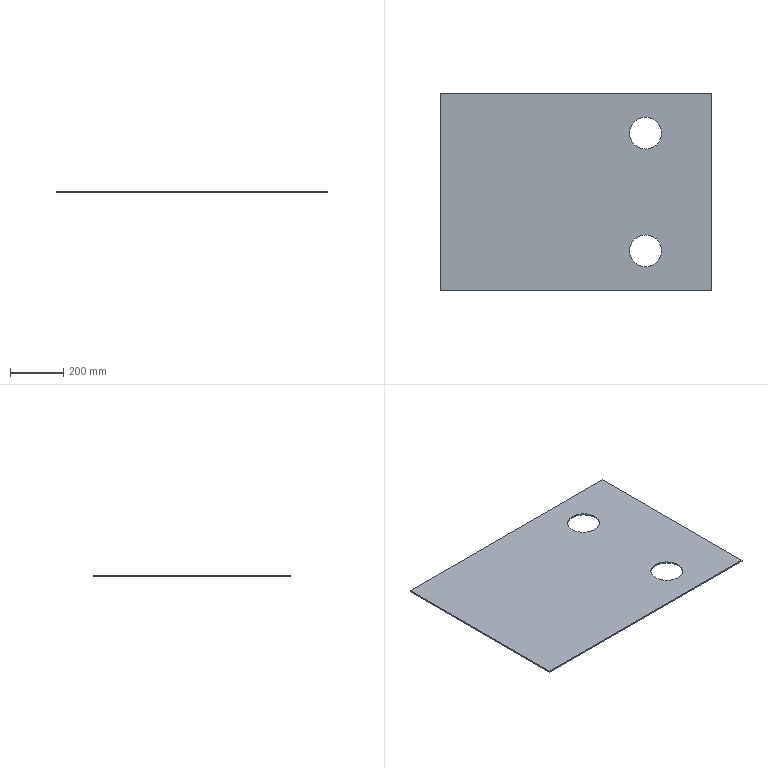Part | SolidWorks | features BaseBody 1 | 1 solid | 10 faces | box 1023 x 743 x 5 mm | volume 3687348 mm3 | plane 6 | cylinder 4 | commonest cylinder face diameters 120 x4
STEP:
#1=CARTESIAN_POINT('',(-250.,653.,5.));
#2=VERTEX_POINT('',#1);
#3=CARTESIAN_POINT('',(-250.,533.,5.));
#4=VERTEX_POINT('',#3);
#5=CARTESIAN_POINT('',(-250.,593.,5.));
#6=DIRECTION('',(0.,0.,1.));
#7=DIRECTION('',(0.,1.,0.));
#8=AXIS2_PLACEMENT_3D('',#5,#6,#7);
#9=CIRCLE('',#8,60.);
#10=EDGE_CURVE('',#2,#4,#9,.T.);
#11=ORIENTED_EDGE('',*,*,#10,.T.);
#12=CARTESIAN_POINT('',(-250.,533.,0.));
#13=VERTEX_POINT('',#12);
#14=CARTESIAN_POINT('',(-250.,533.,5.));
#15=DIRECTION('',(0.,0.,-1.));
#16=VECTOR('',#15,1000.);
#17=LINE('',#14,#16);
#18=EDGE_CURVE('',#4,#13,#17,.T.);
#19=ORIENTED_EDGE('',*,*,#18,.T.);
#20=CARTESIAN_POINT('',(-250.,653.,0.));
#21=VERTEX_POINT('',#20);
#22=CARTESIAN_POINT('',(-250.,593.,0.));
#23=DIRECTION('',(0.,0.,-1.));
#24=DIRECTION('',(0.,1.,0.));
#25=AXIS2_PLACEMENT_3D('',#22,#23,#24);
#26=CIRCLE('',#25,60.);
#27=EDGE_CURVE('',#13,#21,#26,.T.);
#28=ORIENTED_EDGE('',*,*,#27,.T.);
#29=CARTESIAN_POINT('',(-250.,653.,5.));
#30=DIRECTION('',(0.,0.,-1.));
#31=VECTOR('',#30,1000.);
#32=LINE('',#29,#31);
#33=EDGE_CURVE('',#2,#21,#32,.T.);
#34=ORIENTED_EDGE('',*,*,#33,.F.);
#35=EDGE_LOOP('',(#11,#19,#28,#34));
#36=FACE_OUTER_BOUND('',#35,.T.);
#37=CARTESIAN_POINT('',(-250.,593.,5.));
#38=DIRECTION('',(0.,0.,-1.));
#39=DIRECTION('',(0.,1.,0.));
#40=AXIS2_PLACEMENT_3D('',#37,#38,#39);
#41=CYLINDRICAL_SURFACE('',#40,60.);
#42=ADVANCED_FACE('',(#36),#41,.F.);
#43=CARTESIAN_POINT('',(-250.,90.,5.));
#44=VERTEX_POINT('',#43);
#45=CARTESIAN_POINT('',(-250.,210.,5.));
#46=VERTEX_POINT('',#45);
#47=CARTESIAN_POINT('',(-250.,150.,5.));
#48=DIRECTION('',(0.,0.,-1.));
#49=DIRECTION('',(0.,1.,0.));
#50=AXIS2_PLACEMENT_3D('',#47,#48,#49);
#51=CIRCLE('',#50,60.);
#52=EDGE_CURVE('',#44,#46,#51,.T.);
#53=ORIENTED_EDGE('',*,*,#52,.F.);
#54=CARTESIAN_POINT('',(-250.,90.,0.));
#55=VERTEX_POINT('',#54);
#56=CARTESIAN_POINT('',(-250.,90.,5.));
#57=DIRECTION('',(0.,0.,-1.));
#58=VECTOR('',#57,1000.);
#59=LINE('',#56,#58);
#60=EDGE_CURVE('',#44,#55,#59,.T.);
#61=ORIENTED_EDGE('',*,*,#60,.T.);
#62=CARTESIAN_POINT('',(-250.,210.,0.));
#63=VERTEX_POINT('',#62);
#64=CARTESIAN_POINT('',(-250.,150.,0.));
#65=DIRECTION('',(0.,0.,-1.));
#66=DIRECTION('',(0.,1.,0.));
#67=AXIS2_PLACEMENT_3D('',#64,#65,#66);
#68=CIRCLE('',#67,60.);
#69=EDGE_CURVE('',#55,#63,#68,.T.);
#70=ORIENTED_EDGE('',*,*,#69,.T.);
#71=CARTESIAN_POINT('',(-250.,210.,5.));
#72=DIRECTION('',(0.,0.,-1.));
#73=VECTOR('',#72,1000.);
#74=LINE('',#71,#73);
#75=EDGE_CURVE('',#46,#63,#74,.T.);
#76=ORIENTED_EDGE('',*,*,#75,.F.);
#77=EDGE_LOOP('',(#53,#61,#70,#76));
#78=FACE_OUTER_BOUND('',#77,.T.);
#79=CARTESIAN_POINT('',(-250.,150.,5.));
#80=DIRECTION('',(0.,0.,-1.));
#81=DIRECTION('',(0.,1.,0.));
#82=AXIS2_PLACEMENT_3D('',#79,#80,#81);
#83=CYLINDRICAL_SURFACE('',#82,60.);
#84=ADVANCED_FACE('',(#78),#83,.F.);
#85=ORIENTED_EDGE('',*,*,#18,.F.);
#86=CARTESIAN_POINT('',(-250.,593.,5.));
#87=DIRECTION('',(0.,0.,1.));
#88=DIRECTION('',(0.,1.,0.));
#89=AXIS2_PLACEMENT_3D('',#86,#87,#88);
#90=CIRCLE('',#89,60.);
#91=EDGE_CURVE('',#4,#2,#90,.T.);
#92=ORIENTED_EDGE('',*,*,#91,.T.);
#93=ORIENTED_EDGE('',*,*,#33,.T.);
#94=CARTESIAN_POINT('',(-250.,593.,0.));
#95=DIRECTION('',(0.,0.,-1.));
#96=DIRECTION('',(0.,1.,0.));
#97=AXIS2_PLACEMENT_3D('',#94,#95,#96);
#98=CIRCLE('',#97,60.);
#99=EDGE_CURVE('',#21,#13,#98,.T.);
#100=ORIENTED_EDGE('',*,*,#99,.T.);
#101=EDGE_LOOP('',(#85,#92,#93,#100));
#102=FACE_OUTER_BOUND('',#101,.T.);
#103=CARTESIAN_POINT('',(-250.,593.,5.));
#104=DIRECTION('',(0.,0.,-1.));
#105=DIRECTION('',(0.,1.,0.));
#106=AXIS2_PLACEMENT_3D('',#103,#104,#105);
#107=CYLINDRICAL_SURFACE('',#106,60.);
#108=ADVANCED_FACE('',(#102),#107,.F.);
#109=CARTESIAN_POINT('',(-250.,150.,0.));
#110=DIRECTION('',(0.,0.,-1.));
#111=DIRECTION('',(0.,1.,0.));
#112=AXIS2_PLACEMENT_3D('',#109,#110,#111);
#113=CIRCLE('',#112,60.);
#114=EDGE_CURVE('',#63,#55,#113,.T.);
#115=ORIENTED_EDGE('',*,*,#114,.F.);
#116=ORIENTED_EDGE('',*,*,#69,.F.);
#117=EDGE_LOOP('',(#115,#116));
#118=FACE_BOUND('',#117,.T.);
#119=ORIENTED_EDGE('',*,*,#99,.F.);
#120=ORIENTED_EDGE('',*,*,#27,.F.);
#121=EDGE_LOOP('',(#119,#120));
#122=FACE_BOUND('',#121,.T.);
#123=CARTESIAN_POINT('',(-1023.,0.,0.));
#124=VERTEX_POINT('',#123);
#125=CARTESIAN_POINT('',(0.,0.,0.));
#126=VERTEX_POINT('',#125);
#127=CARTESIAN_POINT('',(-511.5,0.,0.));
#128=DIRECTION('',(1.,0.,0.));
#129=VECTOR('',#128,1000.);
#130=LINE('',#127,#129);
#131=EDGE_CURVE('',#124,#126,#130,.T.);
#132=ORIENTED_EDGE('',*,*,#131,.F.);
#133=CARTESIAN_POINT('',(-1023.,743.,0.));
#134=VERTEX_POINT('',#133);
#135=CARTESIAN_POINT('',(-1023.,371.5,0.));
#136=DIRECTION('',(0.,-1.,0.));
#137=VECTOR('',#136,1000.);
#138=LINE('',#135,#137);
#139=EDGE_CURVE('',#134,#124,#138,.T.);
#140=ORIENTED_EDGE('',*,*,#139,.F.);
#141=CARTESIAN_POINT('',(0.,743.,0.));
#142=VERTEX_POINT('',#141);
#143=CARTESIAN_POINT('',(-511.5,743.,0.));
#144=DIRECTION('',(-1.,0.,0.));
#145=VECTOR('',#144,1000.);
#146=LINE('',#143,#145);
#147=EDGE_CURVE('',#142,#134,#146,.T.);
#148=ORIENTED_EDGE('',*,*,#147,.F.);
#149=CARTESIAN_POINT('',(0.,371.5,0.));
#150=DIRECTION('',(0.,1.,0.));
#151=VECTOR('',#150,1000.);
#152=LINE('',#149,#151);
#153=EDGE_CURVE('',#126,#142,#152,.T.);
#154=ORIENTED_EDGE('',*,*,#153,.F.);
#155=EDGE_LOOP('',(#132,#140,#148,#154));
#156=FACE_OUTER_BOUND('',#155,.T.);
#157=CARTESIAN_POINT('',(-1023.,0.,0.));
#158=DIRECTION('',(0.,0.,1.));
#159=DIRECTION('',(1.,0.,0.));
#160=AXIS2_PLACEMENT_3D('',#157,#158,#159);
#161=PLANE('',#160);
#162=ADVANCED_FACE('',(#118,#122,#156),#161,.F.);
#163=CARTESIAN_POINT('',(-250.,150.,5.));
#164=DIRECTION('',(0.,0.,-1.));
#165=DIRECTION('',(0.,1.,0.));
#166=AXIS2_PLACEMENT_3D('',#163,#164,#165);
#167=CIRCLE('',#166,60.);
#168=EDGE_CURVE('',#46,#44,#167,.T.);
#169=ORIENTED_EDGE('',*,*,#168,.T.);
#170=ORIENTED_EDGE('',*,*,#52,.T.);
#171=EDGE_LOOP('',(#169,#170));
#172=FACE_BOUND('',#171,.T.);
#173=ORIENTED_EDGE('',*,*,#10,.F.);
#174=ORIENTED_EDGE('',*,*,#91,.F.);
#175=EDGE_LOOP('',(#173,#174));
#176=FACE_BOUND('',#175,.T.);
#177=CARTESIAN_POINT('',(-1023.,743.,5.));
#178=VERTEX_POINT('',#177);
#179=CARTESIAN_POINT('',(-1023.,0.,5.));
#180=VERTEX_POINT('',#179);
#181=CARTESIAN_POINT('',(-1023.,371.5,5.));
#182=DIRECTION('',(0.,-1.,0.));
#183=VECTOR('',#182,1000.);
#184=LINE('',#181,#183);
#185=EDGE_CURVE('',#178,#180,#184,.T.);
#186=ORIENTED_EDGE('',*,*,#185,.T.);
#187=CARTESIAN_POINT('',(0.,0.,5.));
#188=VERTEX_POINT('',#187);
#189=CARTESIAN_POINT('',(-511.5,0.,5.));
#190=DIRECTION('',(1.,0.,0.));
#191=VECTOR('',#190,1000.);
#192=LINE('',#189,#191);
#193=EDGE_CURVE('',#180,#188,#192,.T.);
#194=ORIENTED_EDGE('',*,*,#193,.T.);
#195=CARTESIAN_POINT('',(0.,743.,5.));
#196=VERTEX_POINT('',#195);
#197=CARTESIAN_POINT('',(0.,371.5,5.));
#198=DIRECTION('',(0.,1.,0.));
#199=VECTOR('',#198,1000.);
#200=LINE('',#197,#199);
#201=EDGE_CURVE('',#188,#196,#200,.T.);
#202=ORIENTED_EDGE('',*,*,#201,.T.);
#203=CARTESIAN_POINT('',(-511.5,743.,5.));
#204=DIRECTION('',(-1.,0.,0.));
#205=VECTOR('',#204,1000.);
#206=LINE('',#203,#205);
#207=EDGE_CURVE('',#196,#178,#206,.T.);
#208=ORIENTED_EDGE('',*,*,#207,.T.);
#209=EDGE_LOOP('',(#186,#194,#202,#208));
#210=FACE_OUTER_BOUND('',#209,.T.);
#211=CARTESIAN_POINT('',(-1023.,0.,5.));
#212=DIRECTION('',(0.,0.,1.));
#213=DIRECTION('',(1.,0.,0.));
#214=AXIS2_PLACEMENT_3D('',#211,#212,#213);
#215=PLANE('',#214);
#216=ADVANCED_FACE('',(#172,#176,#210),#215,.T.);
#217=ORIENTED_EDGE('',*,*,#60,.F.);
#218=ORIENTED_EDGE('',*,*,#168,.F.);
#219=ORIENTED_EDGE('',*,*,#75,.T.);
#220=ORIENTED_EDGE('',*,*,#114,.T.);
#221=EDGE_LOOP('',(#217,#218,#219,#220));
#222=FACE_OUTER_BOUND('',#221,.T.);
#223=CARTESIAN_POINT('',(-250.,150.,5.));
#224=DIRECTION('',(0.,0.,-1.));
#225=DIRECTION('',(0.,1.,0.));
#226=AXIS2_PLACEMENT_3D('',#223,#224,#225);
#227=CYLINDRICAL_SURFACE('',#226,60.);
#228=ADVANCED_FACE('',(#222),#227,.F.);
#229=CARTESIAN_POINT('',(0.,743.,2.5));
#230=DIRECTION('',(0.,0.,-1.));
#231=VECTOR('',#230,1000.);
#232=LINE('',#229,#231);
#233=EDGE_CURVE('',#196,#142,#232,.T.);
#234=ORIENTED_EDGE('',*,*,#233,.F.);
#235=ORIENTED_EDGE('',*,*,#201,.F.);
#236=CARTESIAN_POINT('',(0.,0.,2.5));
#237=DIRECTION('',(0.,0.,1.));
#238=VECTOR('',#237,1000.);
#239=LINE('',#236,#238);
#240=EDGE_CURVE('',#126,#188,#239,.T.);
#241=ORIENTED_EDGE('',*,*,#240,.F.);
#242=ORIENTED_EDGE('',*,*,#153,.T.);
#243=EDGE_LOOP('',(#234,#235,#241,#242));
#244=FACE_OUTER_BOUND('',#243,.T.);
#245=CARTESIAN_POINT('',(0.,0.,0.));
#246=DIRECTION('',(-1.,0.,0.));
#247=DIRECTION('',(0.,0.,1.));
#248=AXIS2_PLACEMENT_3D('',#245,#246,#247);
#249=PLANE('',#248);
#250=ADVANCED_FACE('',(#244),#249,.F.);
#251=ORIENTED_EDGE('',*,*,#240,.T.);
#252=ORIENTED_EDGE('',*,*,#193,.F.);
#253=CARTESIAN_POINT('',(-1023.,0.,2.5));
#254=DIRECTION('',(0.,0.,1.));
#255=VECTOR('',#254,1000.);
#256=LINE('',#253,#255);
#257=EDGE_CURVE('',#124,#180,#256,.T.);
#258=ORIENTED_EDGE('',*,*,#257,.F.);
#259=ORIENTED_EDGE('',*,*,#131,.T.);
#260=EDGE_LOOP('',(#251,#252,#258,#259));
#261=FACE_OUTER_BOUND('',#260,.T.);
#262=CARTESIAN_POINT('',(0.,0.,0.));
#263=DIRECTION('',(0.,1.,0.));
#264=DIRECTION('',(-1.,0.,0.));
#265=AXIS2_PLACEMENT_3D('',#262,#263,#264);
#266=PLANE('',#265);
#267=ADVANCED_FACE('',(#261),#266,.F.);
#268=ORIENTED_EDGE('',*,*,#257,.T.);
#269=ORIENTED_EDGE('',*,*,#185,.F.);
#270=CARTESIAN_POINT('',(-1023.,743.,2.5));
#271=DIRECTION('',(0.,0.,1.));
#272=VECTOR('',#271,1000.);
#273=LINE('',#270,#272);
#274=EDGE_CURVE('',#134,#178,#273,.T.);
#275=ORIENTED_EDGE('',*,*,#274,.F.);
#276=ORIENTED_EDGE('',*,*,#139,.T.);
#277=EDGE_LOOP('',(#268,#269,#275,#276));
#278=FACE_OUTER_BOUND('',#277,.T.);
#279=CARTESIAN_POINT('',(-1023.,0.,5.));
#280=DIRECTION('',(1.,0.,0.));
#281=DIRECTION('',(0.,0.,-1.));
#282=AXIS2_PLACEMENT_3D('',#279,#280,#281);
#283=PLANE('',#282);
#284=ADVANCED_FACE('',(#278),#283,.F.);
#285=ORIENTED_EDGE('',*,*,#274,.T.);
#286=ORIENTED_EDGE('',*,*,#207,.F.);
#287=ORIENTED_EDGE('',*,*,#233,.T.);
#288=ORIENTED_EDGE('',*,*,#147,.T.);
#289=EDGE_LOOP('',(#285,#286,#287,#288));
#290=FACE_OUTER_BOUND('',#289,.T.);
#291=CARTESIAN_POINT('',(-1023.,743.,0.));
#292=DIRECTION('',(0.,-1.,0.));
#293=DIRECTION('',(1.,0.,0.));
#294=AXIS2_PLACEMENT_3D('',#291,#292,#293);
#295=PLANE('',#294);
#296=ADVANCED_FACE('',(#290),#295,.F.);
#297=CLOSED_SHELL('',(#42,#84,#108,#162,#216,#228,#250,#267,#284,#296));
#298=MANIFOLD_SOLID_BREP('',#297);
#299=CARTESIAN_POINT('',(0.,0.,0.));
#300=DIRECTION('',(0.,0.,1.));
#301=DIRECTION('',(1.,0.,0.));
#302=AXIS2_PLACEMENT_3D('',#299,#300,#301);
#303=(LENGTH_UNIT()NAMED_UNIT(*)SI_UNIT(.MILLI.,.METRE.));
#304=UNCERTAINTY_MEASURE_WITH_UNIT(LENGTH_MEASURE(0.00001),#303,'','');
#305=(NAMED_UNIT(*)PLANE_ANGLE_UNIT()SI_UNIT($,.RADIAN.));
#306=(NAMED_UNIT(*)SI_UNIT($,.STERADIAN.)SOLID_ANGLE_UNIT());
#307=(GEOMETRIC_REPRESENTATION_CONTEXT(3)GLOBAL_UNCERTAINTY_ASSIGNED_CONTEXT((#304))GLOBAL_UNIT_ASSIGNED_CONTEXT((#303,#305,#306))REPRESENTATION_CONTEXT('',''));
#308=ADVANCED_BREP_SHAPE_REPRESENTATION('',(#298,#302),#307);